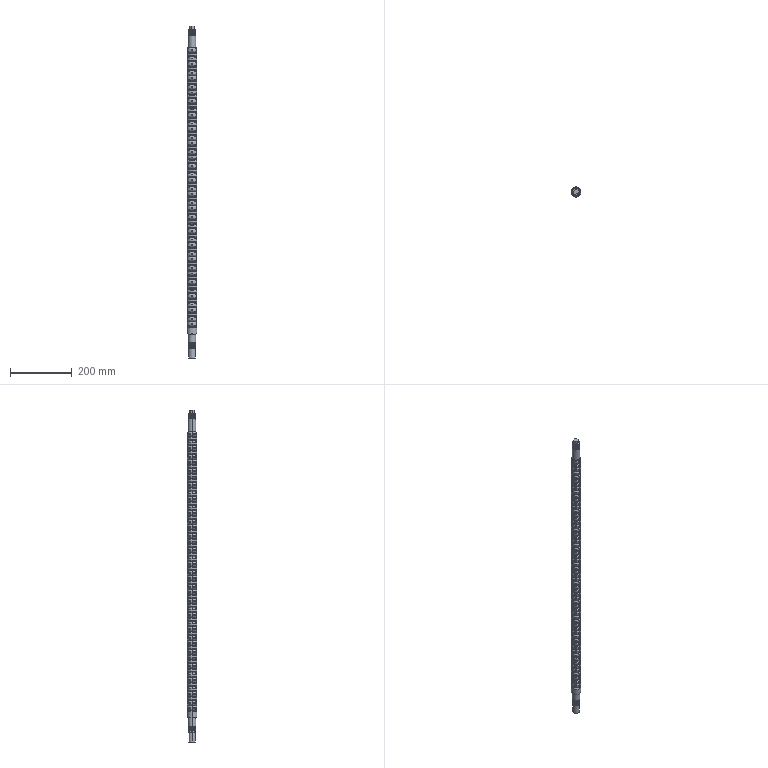Part | STEP file | 400V80 Z-Axis Lead Screw | 1 solid | 736 faces | box 32 x 32 x 1073 mm | volume 695991 mm3 | cylinder 252 | spline 242 | plane 134 | cone 108 | commonest cylinder face diameters 26 x122 32 x122 25 x4 22 x2 24 x2